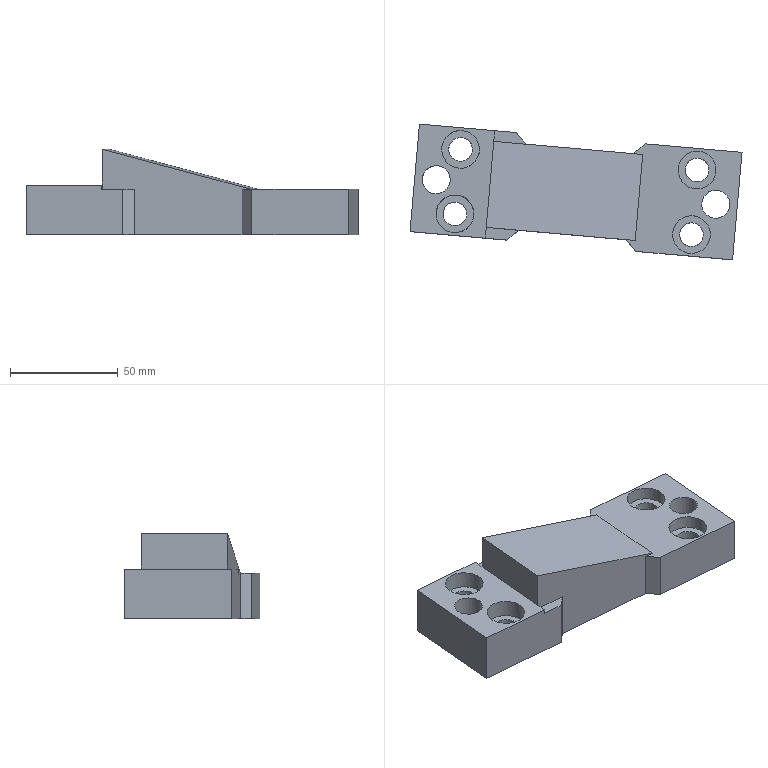Part | NX | features solid 2 | 1 solid | 35 faces | box 153.787 x 62.883 x 39.56 mm | volume 156886 mm3 | plane 25 | cylinder 10 | commonest cylinder face diameters 11 x4 17.5 x4 13 x2
STEP:
#1=CARTESIAN_POINT('',(-568.768,325.811,-44.));
#2=VERTEX_POINT('',#1);
#3=CARTESIAN_POINT('',(-553.825,324.504,-44.));
#4=VERTEX_POINT('',#3);
#5=CARTESIAN_POINT('',(-568.768,325.811,-44.));
#6=DIRECTION('',(0.9962,-0.08716,0.));
#7=VECTOR('',#6,1000.);
#8=LINE('',#5,#7);
#9=EDGE_CURVE('',#2,#4,#8,.T.);
#10=ORIENTED_EDGE('',*,*,#9,.T.);
#11=CARTESIAN_POINT('',(-558.37,329.921,-44.));
#12=VERTEX_POINT('',#11);
#13=CARTESIAN_POINT('',(-553.825,324.504,-44.));
#14=DIRECTION('',(-0.6428,0.766,0.));
#15=VECTOR('',#14,1000.);
#16=LINE('',#13,#15);
#17=EDGE_CURVE('',#4,#12,#16,.T.);
#18=ORIENTED_EDGE('',*,*,#17,.T.);
#19=CARTESIAN_POINT('',(-568.332,330.792,-44.));
#20=VERTEX_POINT('',#19);
#21=CARTESIAN_POINT('',(-603.199,333.843,-44.));
#22=DIRECTION('',(0.9962,-0.08716,0.));
#23=VECTOR('',#22,1000.);
#24=LINE('',#21,#23);
#25=EDGE_CURVE('',#20,#12,#24,.T.);
#26=ORIENTED_EDGE('',*,*,#25,.F.);
#27=CARTESIAN_POINT('',(-572.69,280.982,-44.));
#28=DIRECTION('',(0.08716,0.9962,0.));
#29=VECTOR('',#28,1000.);
#30=LINE('',#27,#29);
#31=EDGE_CURVE('',#2,#20,#30,.T.);
#32=ORIENTED_EDGE('',*,*,#31,.F.);
#33=EDGE_LOOP('',(#10,#18,#26,#32));
#34=FACE_BOUND('',#33,.T.);
#35=CARTESIAN_POINT('',(-607.557,284.033,-44.));
#36=DIRECTION('',(0.,0.,-1.));
#37=DIRECTION('',(-0.08716,-0.9962,0.));
#38=AXIS2_PLACEMENT_3D('',#35,#36,#37);
#39=PLANE('',#38);
#40=ADVANCED_FACE('',(#34),#39,.F.);
#41=CARTESIAN_POINT('',(-572.69,280.982,-44.));
#42=VERTEX_POINT('',#41);
#43=CARTESIAN_POINT('',(-572.254,285.963,-44.));
#44=VERTEX_POINT('',#43);
#45=CARTESIAN_POINT('',(-572.69,280.982,-44.));
#46=DIRECTION('',(0.08716,0.9962,0.));
#47=VECTOR('',#46,1000.);
#48=LINE('',#45,#47);
#49=EDGE_CURVE('',#42,#44,#48,.T.);
#50=ORIENTED_EDGE('',*,*,#49,.F.);
#51=CARTESIAN_POINT('',(-562.728,280.111,-44.));
#52=VERTEX_POINT('',#51);
#53=CARTESIAN_POINT('',(-607.557,284.033,-44.));
#54=DIRECTION('',(0.9962,-0.08716,0.));
#55=VECTOR('',#54,1000.);
#56=LINE('',#53,#55);
#57=EDGE_CURVE('',#42,#52,#56,.T.);
#58=ORIENTED_EDGE('',*,*,#57,.T.);
#59=CARTESIAN_POINT('',(-557.311,284.656,-44.));
#60=VERTEX_POINT('',#59);
#61=CARTESIAN_POINT('',(-562.728,280.111,-44.));
#62=DIRECTION('',(0.766,0.6428,0.));
#63=VECTOR('',#62,1000.);
#64=LINE('',#61,#63);
#65=EDGE_CURVE('',#52,#60,#64,.T.);
#66=ORIENTED_EDGE('',*,*,#65,.T.);
#67=CARTESIAN_POINT('',(-572.254,285.963,-44.));
#68=DIRECTION('',(0.9962,-0.08716,0.));
#69=VECTOR('',#68,1000.);
#70=LINE('',#67,#69);
#71=EDGE_CURVE('',#44,#60,#70,.T.);
#72=ORIENTED_EDGE('',*,*,#71,.F.);
#73=EDGE_LOOP('',(#50,#58,#66,#72));
#74=FACE_BOUND('',#73,.T.);
#75=CARTESIAN_POINT('',(-607.557,284.033,-44.));
#76=DIRECTION('',(0.,0.,-1.));
#77=DIRECTION('',(-0.08716,-0.9962,0.));
#78=AXIS2_PLACEMENT_3D('',#75,#76,#77);
#79=PLANE('',#78);
#80=ADVANCED_FACE('',(#74),#79,.F.);
#81=ORIENTED_EDGE('',*,*,#31,.T.);
#82=CARTESIAN_POINT('',(-568.332,330.792,-42.));
#83=VERTEX_POINT('',#82);
#84=CARTESIAN_POINT('',(-568.332,330.792,-44.));
#85=DIRECTION('',(0.,0.,-1.));
#86=VECTOR('',#85,1000.);
#87=LINE('',#84,#86);
#88=EDGE_CURVE('',#83,#20,#87,.T.);
#89=ORIENTED_EDGE('',*,*,#88,.F.);
#90=CARTESIAN_POINT('',(-568.768,325.811,-42.));
#91=VERTEX_POINT('',#90);
#92=CARTESIAN_POINT('',(-572.69,280.982,-42.));
#93=DIRECTION('',(0.08716,0.9962,0.));
#94=VECTOR('',#93,1000.);
#95=LINE('',#92,#94);
#96=EDGE_CURVE('',#91,#83,#95,.T.);
#97=ORIENTED_EDGE('',*,*,#96,.F.);
#98=CARTESIAN_POINT('',(-568.768,325.811,-25.44));
#99=DIRECTION('',(0.,0.,-1.));
#100=VECTOR('',#99,1000.);
#101=LINE('',#98,#100);
#102=EDGE_CURVE('',#91,#2,#101,.T.);
#103=ORIENTED_EDGE('',*,*,#102,.T.);
#104=EDGE_LOOP('',(#81,#89,#97,#103));
#105=FACE_BOUND('',#104,.T.);
#106=CARTESIAN_POINT('',(-572.69,280.982,-25.44));
#107=DIRECTION('',(0.9962,-0.08716,0.));
#108=DIRECTION('',(-0.08716,-0.9962,0.));
#109=AXIS2_PLACEMENT_3D('',#106,#107,#108);
#110=PLANE('',#109);
#111=ADVANCED_FACE('',(#105),#110,.T.);
#112=CARTESIAN_POINT('',(-468.463,281.902,-44.));
#113=VERTEX_POINT('',#112);
#114=CARTESIAN_POINT('',(-477.18,282.665,-44.));
#115=DIRECTION('',(0.,0.,-1.));
#116=DIRECTION('',(0.9962,-0.08716,0.));
#117=AXIS2_PLACEMENT_3D('',#114,#115,#116);
#118=CIRCLE('',#117,8.75);
#119=EDGE_CURVE('',#113,#113,#118,.T.);
#120=ORIENTED_EDGE('',*,*,#119,.T.);
#121=EDGE_LOOP('',(#120));
#122=FACE_BOUND('',#121,.T.);
#123=CARTESIAN_POINT('',(-507.502,280.298,-44.));
#124=VERTEX_POINT('',#123);
#125=CARTESIAN_POINT('',(-502.956,274.882,-44.));
#126=VERTEX_POINT('',#125);
#127=CARTESIAN_POINT('',(-507.502,280.298,-44.));
#128=DIRECTION('',(0.6428,-0.766,0.));
#129=VECTOR('',#128,1000.);
#130=LINE('',#127,#129);
#131=EDGE_CURVE('',#124,#126,#130,.T.);
#132=ORIENTED_EDGE('',*,*,#131,.T.);
#133=CARTESIAN_POINT('',(-458.128,270.96,-44.));
#134=VERTEX_POINT('',#133);
#135=CARTESIAN_POINT('',(-502.956,274.882,-44.));
#136=DIRECTION('',(0.9962,-0.08716,0.));
#137=VECTOR('',#136,1000.);
#138=LINE('',#135,#137);
#139=EDGE_CURVE('',#126,#134,#138,.T.);
#140=ORIENTED_EDGE('',*,*,#139,.T.);
#141=CARTESIAN_POINT('',(-453.77,320.769,-44.));
#142=VERTEX_POINT('',#141);
#143=CARTESIAN_POINT('',(-458.128,270.96,-44.));
#144=DIRECTION('',(0.08716,0.9962,0.));
#145=VECTOR('',#144,1000.);
#146=LINE('',#143,#145);
#147=EDGE_CURVE('',#134,#142,#146,.T.);
#148=ORIENTED_EDGE('',*,*,#147,.T.);
#149=CARTESIAN_POINT('',(-498.599,324.691,-44.));
#150=VERTEX_POINT('',#149);
#151=CARTESIAN_POINT('',(-498.599,324.691,-44.));
#152=DIRECTION('',(0.9962,-0.08716,0.));
#153=VECTOR('',#152,1000.);
#154=LINE('',#151,#153);
#155=EDGE_CURVE('',#150,#142,#154,.T.);
#156=ORIENTED_EDGE('',*,*,#155,.F.);
#157=CARTESIAN_POINT('',(-504.015,320.146,-44.));
#158=VERTEX_POINT('',#157);
#159=CARTESIAN_POINT('',(-504.015,320.146,-44.));
#160=DIRECTION('',(0.766,0.6428,0.));
#161=VECTOR('',#160,1000.);
#162=LINE('',#159,#161);
#163=EDGE_CURVE('',#158,#150,#162,.T.);
#164=ORIENTED_EDGE('',*,*,#163,.F.);
#165=CARTESIAN_POINT('',(-499.764,319.774,-44.));
#166=VERTEX_POINT('',#165);
#167=CARTESIAN_POINT('',(-568.768,325.811,-44.));
#168=DIRECTION('',(0.9962,-0.08716,0.));
#169=VECTOR('',#168,1000.);
#170=LINE('',#167,#169);
#171=EDGE_CURVE('',#158,#166,#170,.T.);
#172=ORIENTED_EDGE('',*,*,#171,.T.);
#173=CARTESIAN_POINT('',(-503.25,279.926,-44.));
#174=VERTEX_POINT('',#173);
#175=CARTESIAN_POINT('',(-503.25,279.926,-44.));
#176=DIRECTION('',(0.08716,0.9962,0.));
#177=VECTOR('',#176,1000.);
#178=LINE('',#175,#177);
#179=EDGE_CURVE('',#174,#166,#178,.T.);
#180=ORIENTED_EDGE('',*,*,#179,.F.);
#181=CARTESIAN_POINT('',(-572.254,285.963,-44.));
#182=DIRECTION('',(0.9962,-0.08716,0.));
#183=VECTOR('',#182,1000.);
#184=LINE('',#181,#183);
#185=EDGE_CURVE('',#124,#174,#184,.T.);
#186=ORIENTED_EDGE('',*,*,#185,.F.);
#187=EDGE_LOOP('',(#132,#140,#148,#156,#164,#172,#180,#186));
#188=FACE_BOUND('',#187,.T.);
#189=CARTESIAN_POINT('',(-459.435,296.169,-44.));
#190=VERTEX_POINT('',#189);
#191=CARTESIAN_POINT('',(-465.911,296.736,-44.));
#192=DIRECTION('',(0.,0.,-1.));
#193=DIRECTION('',(0.9962,-0.08716,0.));
#194=AXIS2_PLACEMENT_3D('',#191,#192,#193);
#195=CIRCLE('',#194,6.5);
#196=EDGE_CURVE('',#190,#190,#195,.T.);
#197=ORIENTED_EDGE('',*,*,#196,.T.);
#198=EDGE_LOOP('',(#197));
#199=FACE_BOUND('',#198,.T.);
#200=CARTESIAN_POINT('',(-465.849,311.788,-44.));
#201=VERTEX_POINT('',#200);
#202=CARTESIAN_POINT('',(-474.565,312.55,-44.));
#203=DIRECTION('',(0.,0.,-1.));
#204=DIRECTION('',(0.9962,-0.08716,0.));
#205=AXIS2_PLACEMENT_3D('',#202,#203,#204);
#206=CIRCLE('',#205,8.75);
#207=EDGE_CURVE('',#201,#201,#206,.T.);
#208=ORIENTED_EDGE('',*,*,#207,.T.);
#209=EDGE_LOOP('',(#208));
#210=FACE_BOUND('',#209,.T.);
#211=CARTESIAN_POINT('',(-607.557,284.033,-44.));
#212=DIRECTION('',(0.,0.,-1.));
#213=DIRECTION('',(-0.08716,-0.9962,0.));
#214=AXIS2_PLACEMENT_3D('',#211,#212,#213);
#215=PLANE('',#214);
#216=ADVANCED_FACE('',(#122,#188,#199,#210),#215,.F.);
#217=CARTESIAN_POINT('',(-469.086,312.071,-65.));
#218=VERTEX_POINT('',#217);
#219=CARTESIAN_POINT('',(-474.565,312.55,-65.));
#220=DIRECTION('',(0.,0.,-1.));
#221=DIRECTION('',(0.9962,-0.08716,0.));
#222=AXIS2_PLACEMENT_3D('',#219,#220,#221);
#223=CIRCLE('',#222,5.5);
#224=EDGE_CURVE('',#218,#218,#223,.T.);
#225=ORIENTED_EDGE('',*,*,#224,.T.);
#226=EDGE_LOOP('',(#225));
#227=FACE_BOUND('',#226,.T.);
#228=CARTESIAN_POINT('',(-474.086,318.03,-50.));
#229=VERTEX_POINT('',#228);
#230=CARTESIAN_POINT('',(-474.565,312.55,-50.));
#231=DIRECTION('',(0.,0.,-1.));
#232=DIRECTION('',(0.08716,0.9962,0.));
#233=AXIS2_PLACEMENT_3D('',#230,#231,#232);
#234=CIRCLE('',#233,5.5);
#235=EDGE_CURVE('',#229,#229,#234,.T.);
#236=ORIENTED_EDGE('',*,*,#235,.F.);
#237=EDGE_LOOP('',(#236));
#238=FACE_BOUND('',#237,.T.);
#239=CARTESIAN_POINT('',(-474.565,312.55,-44.));
#240=DIRECTION('',(0.,0.,-1.));
#241=DIRECTION('',(-0.08716,-0.9962,0.));
#242=AXIS2_PLACEMENT_3D('',#239,#240,#241);
#243=CYLINDRICAL_SURFACE('',#242,5.5);
#244=ADVANCED_FACE('',(#227,#238),#243,.F.);
#245=CARTESIAN_POINT('',(-471.701,282.185,-65.));
#246=VERTEX_POINT('',#245);
#247=CARTESIAN_POINT('',(-477.18,282.665,-65.));
#248=DIRECTION('',(0.,0.,-1.));
#249=DIRECTION('',(0.9962,-0.08716,0.));
#250=AXIS2_PLACEMENT_3D('',#247,#248,#249);
#251=CIRCLE('',#250,5.5);
#252=EDGE_CURVE('',#246,#246,#251,.T.);
#253=ORIENTED_EDGE('',*,*,#252,.T.);
#254=EDGE_LOOP('',(#253));
#255=FACE_BOUND('',#254,.T.);
#256=CARTESIAN_POINT('',(-476.701,288.144,-50.));
#257=VERTEX_POINT('',#256);
#258=CARTESIAN_POINT('',(-477.18,282.665,-50.));
#259=DIRECTION('',(0.,0.,-1.));
#260=DIRECTION('',(0.08716,0.9962,0.));
#261=AXIS2_PLACEMENT_3D('',#258,#259,#260);
#262=CIRCLE('',#261,5.5);
#263=EDGE_CURVE('',#257,#257,#262,.T.);
#264=ORIENTED_EDGE('',*,*,#263,.F.);
#265=EDGE_LOOP('',(#264));
#266=FACE_BOUND('',#265,.T.);
#267=CARTESIAN_POINT('',(-477.18,282.665,-44.));
#268=DIRECTION('',(0.,0.,-1.));
#269=DIRECTION('',(-0.08716,-0.9962,0.));
#270=AXIS2_PLACEMENT_3D('',#267,#268,#269);
#271=CYLINDRICAL_SURFACE('',#270,5.5);
#272=ADVANCED_FACE('',(#255,#266),#271,.F.);
#273=CARTESIAN_POINT('',(-603.199,333.843,-65.));
#274=VERTEX_POINT('',#273);
#275=CARTESIAN_POINT('',(-558.37,329.921,-65.));
#276=VERTEX_POINT('',#275);
#277=CARTESIAN_POINT('',(-603.199,333.843,-65.));
#278=DIRECTION('',(0.9962,-0.08716,0.));
#279=VECTOR('',#278,1000.);
#280=LINE('',#277,#279);
#281=EDGE_CURVE('',#274,#276,#280,.T.);
#282=ORIENTED_EDGE('',*,*,#281,.T.);
#283=CARTESIAN_POINT('',(-553.825,324.504,-65.));
#284=VERTEX_POINT('',#283);
#285=CARTESIAN_POINT('',(-553.825,324.504,-65.));
#286=DIRECTION('',(-0.6428,0.766,0.));
#287=VECTOR('',#286,1000.);
#288=LINE('',#285,#287);
#289=EDGE_CURVE('',#284,#276,#288,.T.);
#290=ORIENTED_EDGE('',*,*,#289,.F.);
#291=CARTESIAN_POINT('',(-504.015,320.146,-65.));
#292=VERTEX_POINT('',#291);
#293=CARTESIAN_POINT('',(-553.825,324.504,-65.));
#294=DIRECTION('',(0.9962,-0.08716,0.));
#295=VECTOR('',#294,1000.);
#296=LINE('',#293,#295);
#297=EDGE_CURVE('',#284,#292,#296,.T.);
#298=ORIENTED_EDGE('',*,*,#297,.T.);
#299=CARTESIAN_POINT('',(-498.599,324.691,-65.));
#300=VERTEX_POINT('',#299);
#301=CARTESIAN_POINT('',(-504.015,320.146,-65.));
#302=DIRECTION('',(0.766,0.6428,0.));
#303=VECTOR('',#302,1000.);
#304=LINE('',#301,#303);
#305=EDGE_CURVE('',#292,#300,#304,.T.);
#306=ORIENTED_EDGE('',*,*,#305,.T.);
#307=CARTESIAN_POINT('',(-453.77,320.769,-65.));
#308=VERTEX_POINT('',#307);
#309=CARTESIAN_POINT('',(-498.599,324.691,-65.));
#310=DIRECTION('',(0.9962,-0.08716,0.));
#311=VECTOR('',#310,1000.);
#312=LINE('',#309,#311);
#313=EDGE_CURVE('',#300,#308,#312,.T.);
#314=ORIENTED_EDGE('',*,*,#313,.T.);
#315=CARTESIAN_POINT('',(-458.128,270.96,-65.));
#316=VERTEX_POINT('',#315);
#317=CARTESIAN_POINT('',(-458.128,270.96,-65.));
#318=DIRECTION('',(0.08716,0.9962,0.));
#319=VECTOR('',#318,1000.);
#320=LINE('',#317,#319);
#321=EDGE_CURVE('',#316,#308,#320,.T.);
#322=ORIENTED_EDGE('',*,*,#321,.F.);
#323=CARTESIAN_POINT('',(-502.956,274.882,-65.));
#324=VERTEX_POINT('',#323);
#325=CARTESIAN_POINT('',(-502.956,274.882,-65.));
#326=DIRECTION('',(0.9962,-0.08716,0.));
#327=VECTOR('',#326,1000.);
#328=LINE('',#325,#327);
#329=EDGE_CURVE('',#324,#316,#328,.T.);
#330=ORIENTED_EDGE('',*,*,#329,.F.);
#331=CARTESIAN_POINT('',(-507.502,280.298,-65.));
#332=VERTEX_POINT('',#331);
#333=CARTESIAN_POINT('',(-507.502,280.298,-65.));
#334=DIRECTION('',(0.6428,-0.766,0.));
#335=VECTOR('',#334,1000.);
#336=LINE('',#333,#335);
#337=EDGE_CURVE('',#332,#324,#336,.T.);
#338=ORIENTED_EDGE('',*,*,#337,.F.);
#339=CARTESIAN_POINT('',(-557.311,284.656,-65.));
#340=VERTEX_POINT('',#339);
#341=CARTESIAN_POINT('',(-557.311,284.656,-65.));
#342=DIRECTION('',(0.9962,-0.08716,0.));
#343=VECTOR('',#342,1000.);
#344=LINE('',#341,#343);
#345=EDGE_CURVE('',#340,#332,#344,.T.);
#346=ORIENTED_EDGE('',*,*,#345,.F.);
#347=CARTESIAN_POINT('',(-562.728,280.111,-65.));
#348=VERTEX_POINT('',#347);
#349=CARTESIAN_POINT('',(-562.728,280.111,-65.));
#350=DIRECTION('',(0.766,0.6428,0.));
#351=VECTOR('',#350,1000.);
#352=LINE('',#349,#351);
#353=EDGE_CURVE('',#348,#340,#352,.T.);
#354=ORIENTED_EDGE('',*,*,#353,.F.);
#355=CARTESIAN_POINT('',(-607.557,284.033,-65.));
#356=VERTEX_POINT('',#355);
#357=CARTESIAN_POINT('',(-607.557,284.033,-65.));
#358=DIRECTION('',(0.9962,-0.08716,0.));
#359=VECTOR('',#358,1000.);
#360=LINE('',#357,#359);
#361=EDGE_CURVE('',#356,#348,#360,.T.);
#362=ORIENTED_EDGE('',*,*,#361,.F.);
#363=CARTESIAN_POINT('',(-603.199,333.843,-65.));
#364=DIRECTION('',(-0.08716,-0.9962,0.));
#365=VECTOR('',#364,1000.);
#366=LINE('',#363,#365);
#367=EDGE_CURVE('',#274,#356,#366,.T.);
#368=ORIENTED_EDGE('',*,*,#367,.F.);
#369=EDGE_LOOP('',(#282,#290,#298,#306,#314,#322,#330,#338,#346,#354,#362,#368));
#370=FACE_BOUND('',#369,.T.);
#371=ORIENTED_EDGE('',*,*,#224,.F.);
#372=EDGE_LOOP('',(#371));
#373=FACE_BOUND('',#372,.T.);
#374=ORIENTED_EDGE('',*,*,#252,.F.);
#375=EDGE_LOOP('',(#374));
#376=FACE_BOUND('',#375,.T.);
#377=CARTESIAN_POINT('',(-459.435,296.169,-65.));
#378=VERTEX_POINT('',#377);
#379=CARTESIAN_POINT('',(-465.911,296.736,-65.));
#380=DIRECTION('',(0.,0.,-1.));
#381=DIRECTION('',(0.9962,-0.08716,0.));
#382=AXIS2_PLACEMENT_3D('',#379,#380,#381);
#383=CIRCLE('',#382,6.5);
#384=EDGE_CURVE('',#378,#378,#383,.T.);
#385=ORIENTED_EDGE('',*,*,#384,.F.);
#386=EDGE_LOOP('',(#385));
#387=FACE_BOUND('',#386,.T.);
#388=CARTESIAN_POINT('',(-578.668,321.658,-65.));
#389=VERTEX_POINT('',#388);
#390=CARTESIAN_POINT('',(-584.147,322.138,-65.));
#391=DIRECTION('',(0.,0.,-1.));
#392=DIRECTION('',(0.9962,-0.08716,0.));
#393=AXIS2_PLACEMENT_3D('',#390,#391,#392);
#394=CIRCLE('',#393,5.5);
#395=EDGE_CURVE('',#389,#389,#394,.T.);
#396=ORIENTED_EDGE('',*,*,#395,.F.);
#397=EDGE_LOOP('',(#396));
#398=FACE_BOUND('',#397,.T.);
#399=CARTESIAN_POINT('',(-581.282,291.772,-65.));
#400=VERTEX_POINT('',#399);
#401=CARTESIAN_POINT('',(-586.761,292.252,-65.));
#402=DIRECTION('',(0.,0.,-1.));
#403=DIRECTION('',(0.9962,-0.08716,0.));
#404=AXIS2_PLACEMENT_3D('',#401,#402,#403);
#405=CIRCLE('',#404,5.5);
#406=EDGE_CURVE('',#400,#400,#405,.T.);
#407=ORIENTED_EDGE('',*,*,#406,.F.);
#408=EDGE_LOOP('',(#407));
#409=FACE_BOUND('',#408,.T.);
#410=CARTESIAN_POINT('',(-588.941,307.5,-65.));
#411=VERTEX_POINT('',#410);
#412=CARTESIAN_POINT('',(-595.416,308.066,-65.));
#413=DIRECTION('',(0.,0.,-1.));
#414=DIRECTION('',(0.9962,-0.08716,0.));
#415=AXIS2_PLACEMENT_3D('',#412,#413,#414);
#416=CIRCLE('',#415,6.5);
#417=EDGE_CURVE('',#411,#411,#416,.T.);
#418=ORIENTED_EDGE('',*,*,#417,.F.);
#419=EDGE_LOOP('',(#418));
#420=FACE_BOUND('',#419,.T.);
#421=CARTESIAN_POINT('',(-607.557,284.033,-65.));
#422=DIRECTION('',(0.,0.,-1.));
#423=DIRECTION('',(-0.08716,-0.9962,0.));
#424=AXIS2_PLACEMENT_3D('',#421,#422,#423);
#425=PLANE('',#424);
#426=ADVANCED_FACE('',(#370,#373,#376,#387,#398,#409,#420),#425,.T.);
#427=ORIENTED_EDGE('',*,*,#361,.T.);
#428=CARTESIAN_POINT('',(-562.728,280.111,-44.));
#429=DIRECTION('',(0.,0.,-1.));
#430=VECTOR('',#429,1000.);
#431=LINE('',#428,#430);
#432=EDGE_CURVE('',#52,#348,#431,.T.);
#433=ORIENTED_EDGE('',*,*,#432,.F.);
#434=ORIENTED_EDGE('',*,*,#57,.F.);
#435=CARTESIAN_POINT('',(-572.69,280.982,-42.));
#436=VERTEX_POINT('',#435);
#437=CARTESIAN_POINT('',(-572.69,280.982,-44.));
#438=DIRECTION('',(0.,0.,-1.));
#439=VECTOR('',#438,1000.);
#440=LINE('',#437,#439);
#441=EDGE_CURVE('',#436,#42,#440,.T.);
#442=ORIENTED_EDGE('',*,*,#441,.F.);
#443=CARTESIAN_POINT('',(-607.557,284.033,-42.));
#444=VERTEX_POINT('',#443);
#445=CARTESIAN_POINT('',(-607.557,284.033,-42.));
#446=DIRECTION('',(0.9962,-0.08716,0.));
#447=VECTOR('',#446,1000.);
#448=LINE('',#445,#447);
#449=EDGE_CURVE('',#444,#436,#448,.T.);
#450=ORIENTED_EDGE('',*,*,#449,.F.);
#451=CARTESIAN_POINT('',(-607.557,284.033,-44.));
#452=DIRECTION('',(0.,0.,-1.));
#453=VECTOR('',#452,1000.);
#454=LINE('',#451,#453);
#455=EDGE_CURVE('',#444,#356,#454,.T.);
#456=ORIENTED_EDGE('',*,*,#455,.T.);
#457=EDGE_LOOP('',(#427,#433,#434,#442,#450,#456));
#458=FACE_BOUND('',#457,.T.);
#459=CARTESIAN_POINT('',(-607.557,284.033,-44.));
#460=DIRECTION('',(-0.08716,-0.9962,0.));
#461=DIRECTION('',(-0.9962,0.08716,0.));
#462=AXIS2_PLACEMENT_3D('',#459,#460,#461);
#463=PLANE('',#462);
#464=ADVANCED_FACE('',(#458),#463,.T.);
#465=ORIENTED_EDGE('',*,*,#353,.T.);
#466=CARTESIAN_POINT('',(-557.311,284.656,-44.));
#467=DIRECTION('',(0.,0.,-1.));
#468=VECTOR('',#467,1000.);
#469=LINE('',#466,#468);
#470=EDGE_CURVE('',#60,#340,#469,.T.);
#471=ORIENTED_EDGE('',*,*,#470,.F.);
#472=ORIENTED_EDGE('',*,*,#65,.F.);
#473=ORIENTED_EDGE('',*,*,#432,.T.);
#474=EDGE_LOOP('',(#465,#471,#472,#473));
#475=FACE_BOUND('',#474,.T.);
#476=CARTESIAN_POINT('',(-562.728,280.111,-44.));
#477=DIRECTION('',(0.6428,-0.766,0.));
#478=DIRECTION('',(-0.766,-0.6428,0.));
#479=AXIS2_PLACEMENT_3D('',#476,#477,#478);
#480=PLANE('',#479);
#481=ADVANCED_FACE('',(#475),#480,.T.);
#482=ORIENTED_EDGE('',*,*,#345,.T.);
#483=CARTESIAN_POINT('',(-507.502,280.298,-44.));
#484=DIRECTION('',(0.,0.,-1.));
#485=VECTOR('',#484,1000.);
#486=LINE('',#483,#485);
#487=EDGE_CURVE('',#124,#332,#486,.T.);
#488=ORIENTED_EDGE('',*,*,#487,.F.);
#489=ORIENTED_EDGE('',*,*,#185,.T.);
#490=CARTESIAN_POINT('',(-572.254,285.963,-25.44));
#491=VERTEX_POINT('',#490);
#492=CARTESIAN_POINT('',(-572.254,285.963,-25.44));
#493=DIRECTION('',(0.9623,-0.08419,-0.2588));
#494=VECTOR('',#493,1000.);
#495=LINE('',#492,#494);
#496=EDGE_CURVE('',#491,#174,#495,.T.);
#497=ORIENTED_EDGE('',*,*,#496,.F.);
#498=CARTESIAN_POINT('',(-572.254,285.963,-42.));
#499=VERTEX_POINT('',#498);
#500=CARTESIAN_POINT('',(-572.254,285.963,-25.44));
#501=DIRECTION('',(0.,0.,-1.));
#502=VECTOR('',#501,1000.);
#503=LINE('',#500,#502);
#504=EDGE_CURVE('',#491,#499,#503,.T.);
#505=ORIENTED_EDGE('',*,*,#504,.T.);
#506=CARTESIAN_POINT('',(-572.254,285.963,-25.44));
#507=DIRECTION('',(0.,0.,-1.));
#508=VECTOR('',#507,1000.);
#509=LINE('',#506,#508);
#510=EDGE_CURVE('',#499,#44,#509,.T.);
#511=ORIENTED_EDGE('',*,*,#510,.T.);
#512=ORIENTED_EDGE('',*,*,#71,.T.);
#513=ORIENTED_EDGE('',*,*,#470,.T.);
#514=EDGE_LOOP('',(#482,#488,#489,#497,#505,#511,#512,#513));
#515=FACE_BOUND('',#514,.T.);
#516=CARTESIAN_POINT('',(-557.311,284.656,-44.));
#517=DIRECTION('',(-0.08716,-0.9962,0.));
#518=DIRECTION('',(-0.9962,0.08716,0.));
#519=AXIS2_PLACEMENT_3D('',#516,#517,#518);
#520=PLANE('',#519);
#521=ADVANCED_FACE('',(#515),#520,.T.);
#522=ORIENTED_EDGE('',*,*,#337,.T.);
#523=CARTESIAN_POINT('',(-502.956,274.882,-44.));
#524=DIRECTION('',(0.,0.,-1.));
#525=VECTOR('',#524,1000.);
#526=LINE('',#523,#525);
#527=EDGE_CURVE('',#126,#324,#526,.T.);
#528=ORIENTED_EDGE('',*,*,#527,.F.);
#529=ORIENTED_EDGE('',*,*,#131,.F.);
#530=ORIENTED_EDGE('',*,*,#487,.T.);
#531=EDGE_LOOP('',(#522,#528,#529,#530));
#532=FACE_BOUND('',#531,.T.);
#533=CARTESIAN_POINT('',(-507.502,280.298,-44.));
#534=DIRECTION('',(-0.766,-0.6428,0.));
#535=DIRECTION('',(-0.6428,0.766,0.));
#536=AXIS2_PLACEMENT_3D('',#533,#534,#535);
#537=PLANE('',#536);
#538=ADVANCED_FACE('',(#532),#537,.T.);
#539=ORIENTED_EDGE('',*,*,#329,.T.);
#540=CARTESIAN_POINT('',(-458.128,270.96,-44.));
#541=DIRECTION('',(0.,0.,-1.));
#542=VECTOR('',#541,1000.);
#543=LINE('',#540,#542);
#544=EDGE_CURVE('',#134,#316,#543,.T.);
#545=ORIENTED_EDGE('',*,*,#544,.F.);
#546=ORIENTED_EDGE('',*,*,#139,.F.);
#547=ORIENTED_EDGE('',*,*,#527,.T.);
#548=EDGE_LOOP('',(#539,#545,#546,#547));
#549=FACE_BOUND('',#548,.T.);
#550=CARTESIAN_POINT('',(-502.956,274.882,-44.));
#551=DIRECTION('',(-0.08716,-0.9962,0.));
#552=DIRECTION('',(-0.9962,0.08716,0.));
#553=AXIS2_PLACEMENT_3D('',#550,#551,#552);
#554=PLANE('',#553);
#555=ADVANCED_FACE('',(#549),#554,.T.);
#556=ORIENTED_EDGE('',*,*,#321,.T.);
#557=CARTESIAN_POINT('',(-453.77,320.769,-44.));
#558=DIRECTION('',(0.,0.,-1.));
#559=VECTOR('',#558,1000.);
#560=LINE('',#557,#559);
#561=EDGE_CURVE('',#142,#308,#560,.T.);
#562=ORIENTED_EDGE('',*,*,#561,.F.);
#563=ORIENTED_EDGE('',*,*,#147,.F.);
#564=ORIENTED_EDGE('',*,*,#544,.T.);
#565=EDGE_LOOP('',(#556,#562,#563,#564));
#566=FACE_BOUND('',#565,.T.);
#567=CARTESIAN_POINT('',(-458.128,270.96,-44.));
#568=DIRECTION('',(0.9962,-0.08716,0.));
#569=DIRECTION('',(-0.08716,-0.9962,0.));
#570=AXIS2_PLACEMENT_3D('',#567,#568,#569);
#571=PLANE('',#570);
#572=ADVANCED_FACE('',(#566),#571,.T.);
#573=ORIENTED_EDGE('',*,*,#313,.F.);
#574=CARTESIAN_POINT('',(-498.599,324.691,-44.));
#575=DIRECTION('',(0.,0.,-1.));
#576=VECTOR('',#575,1000.);
#577=LINE('',#574,#576);
#578=EDGE_CURVE('',#150,#300,#577,.T.);
#579=ORIENTED_EDGE('',*,*,#578,.F.);
#580=ORIENTED_EDGE('',*,*,#155,.T.);
#581=ORIENTED_EDGE('',*,*,#561,.T.);
#582=EDGE_LOOP('',(#573,#579,#580,#581));
#583=FACE_BOUND('',#582,.T.);
#584=CARTESIAN_POINT('',(-498.599,324.691,-44.));
#585=DIRECTION('',(-0.08716,-0.9962,0.));
#586=DIRECTION('',(-0.9962,0.08716,0.));
#587=AXIS2_PLACEMENT_3D('',#584,#585,#586);
#588=PLANE('',#587);
#589=ADVANCED_FACE('',(#583),#588,.F.);
#590=ORIENTED_EDGE('',*,*,#305,.F.);
#591=CARTESIAN_POINT('',(-504.015,320.146,-44.));
#592=DIRECTION('',(0.,0.,-1.));
#593=VECTOR('',#592,1000.);
#594=LINE('',#591,#593);
#595=EDGE_CURVE('',#158,#292,#594,.T.);
#596=ORIENTED_EDGE('',*,*,#595,.F.);
#597=ORIENTED_EDGE('',*,*,#163,.T.);
#598=ORIENTED_EDGE('',*,*,#578,.T.);
#599=EDGE_LOOP('',(#590,#596,#597,#598));
#600=FACE_BOUND('',#599,.T.);
#601=CARTESIAN_POINT('',(-504.015,320.146,-44.));
#602=DIRECTION('',(0.6428,-0.766,0.));
#603=DIRECTION('',(-0.766,-0.6428,0.));
#604=AXIS2_PLACEMENT_3D('',#601,#602,#603);
#605=PLANE('',#604);
#606=ADVANCED_FACE('',(#600),#605,.F.);
#607=ORIENTED_EDGE('',*,*,#297,.F.);
#608=CARTESIAN_POINT('',(-553.825,324.504,-44.));
#609=DIRECTION('',(0.,0.,-1.));
#610=VECTOR('',#609,1000.);
#611=LINE('',#608,#610);
#612=EDGE_CURVE('',#4,#284,#611,.T.);
#613=ORIENTED_EDGE('',*,*,#612,.F.);
#614=ORIENTED_EDGE('',*,*,#9,.F.);
#615=ORIENTED_EDGE('',*,*,#102,.F.);
#616=CARTESIAN_POINT('',(-568.768,325.811,-25.44));
#617=VERTEX_POINT('',#616);
#618=CARTESIAN_POINT('',(-568.768,325.811,-25.44));
#619=DIRECTION('',(0.,0.,-1.));
#620=VECTOR('',#619,1000.);
#621=LINE('',#618,#620);
#622=EDGE_CURVE('',#617,#91,#621,.T.);
#623=ORIENTED_EDGE('',*,*,#622,.F.);
#624=CARTESIAN_POINT('',(-568.768,325.811,-25.44));
#625=DIRECTION('',(0.9623,-0.08419,-0.2588));
#626=VECTOR('',#625,1000.);
#627=LINE('',#624,#626);
#628=EDGE_CURVE('',#617,#166,#627,.T.);
#629=ORIENTED_EDGE('',*,*,#628,.T.);
#630=ORIENTED_EDGE('',*,*,#171,.F.);
#631=ORIENTED_EDGE('',*,*,#595,.T.);
#632=EDGE_LOOP('',(#607,#613,#614,#615,#623,#629,#630,#631));
#633=FACE_BOUND('',#632,.T.);
#634=CARTESIAN_POINT('',(-553.825,324.504,-44.));
#635=DIRECTION('',(-0.08716,-0.9962,0.));
#636=DIRECTION('',(-0.9962,0.08716,0.));
#637=AXIS2_PLACEMENT_3D('',#634,#635,#636);
#638=PLANE('',#637);
#639=ADVANCED_FACE('',(#633),#638,.F.);
#640=ORIENTED_EDGE('',*,*,#289,.T.);
#641=CARTESIAN_POINT('',(-558.37,329.921,-44.));
#642=DIRECTION('',(0.,0.,-1.));
#643=VECTOR('',#642,1000.);
#644=LINE('',#641,#643);
#645=EDGE_CURVE('',#12,#276,#644,.T.);
#646=ORIENTED_EDGE('',*,*,#645,.F.);
#647=ORIENTED_EDGE('',*,*,#17,.F.);
#648=ORIENTED_EDGE('',*,*,#612,.T.);
#649=EDGE_LOOP('',(#640,#646,#647,#648));
#650=FACE_BOUND('',#649,.T.);
#651=CARTESIAN_POINT('',(-553.825,324.504,-44.));
#652=DIRECTION('',(0.766,0.6428,0.));
#653=DIRECTION('',(0.6428,-0.766,0.));
#654=AXIS2_PLACEMENT_3D('',#651,#652,#653);
#655=PLANE('',#654);
#656=ADVANCED_FACE('',(#650),#655,.T.);
#657=ORIENTED_EDGE('',*,*,#25,.T.);
#658=ORIENTED_EDGE('',*,*,#645,.T.);
#659=ORIENTED_EDGE('',*,*,#281,.F.);
#660=CARTESIAN_POINT('',(-603.199,333.843,-42.));
#661=VERTEX_POINT('',#660);
#662=CARTESIAN_POINT('',(-603.199,333.843,-44.));
#663=DIRECTION('',(0.,0.,-1.));
#664=VECTOR('',#663,1000.);
#665=LINE('',#662,#664);
#666=EDGE_CURVE('',#661,#274,#665,.T.);
#667=ORIENTED_EDGE('',*,*,#666,.F.);
#668=CARTESIAN_POINT('',(-603.199,333.843,-42.));
#669=DIRECTION('',(0.9962,-0.08716,0.));
#670=VECTOR('',#669,1000.);
#671=LINE('',#668,#670);
#672=EDGE_CURVE('',#661,#83,#671,.T.);
#673=ORIENTED_EDGE('',*,*,#672,.T.);
#674=ORIENTED_EDGE('',*,*,#88,.T.);
#675=EDGE_LOOP('',(#657,#658,#659,#667,#673,#674));
#676=FACE_BOUND('',#675,.T.);
#677=CARTESIAN_POINT('',(-603.199,333.843,-44.));
#678=DIRECTION('',(-0.08716,-0.9962,0.));
#679=DIRECTION('',(-0.9962,0.08716,0.));
#680=AXIS2_PLACEMENT_3D('',#677,#678,#679);
#681=PLANE('',#680);
#682=ADVANCED_FACE('',(#676),#681,.F.);
#683=ORIENTED_EDGE('',*,*,#196,.F.);
#684=EDGE_LOOP('',(#683));
#685=FACE_BOUND('',#684,.T.);
#686=ORIENTED_EDGE('',*,*,#384,.T.);
#687=EDGE_LOOP('',(#686));
#688=FACE_BOUND('',#687,.T.);
#689=CARTESIAN_POINT('',(-465.911,296.736,-44.));
#690=DIRECTION('',(0.,0.,-1.));
#691=DIRECTION('',(-0.08716,-0.9962,0.));
#692=AXIS2_PLACEMENT_3D('',#689,#690,#691);
#693=CYLINDRICAL_SURFACE('',#692,6.5);
#694=ADVANCED_FACE('',(#685,#688),#693,.F.);
#695=ORIENTED_EDGE('',*,*,#119,.F.);
#696=EDGE_LOOP('',(#695));
#697=FACE_BOUND('',#696,.T.);
#698=CARTESIAN_POINT('',(-468.463,281.902,-50.));
#699=VERTEX_POINT('',#698);
#700=CARTESIAN_POINT('',(-477.18,282.665,-50.));
#701=DIRECTION('',(0.,0.,-1.));
#702=DIRECTION('',(0.9962,-0.08716,0.));
#703=AXIS2_PLACEMENT_3D('',#700,#701,#702);
#704=CIRCLE('',#703,8.75);
#705=EDGE_CURVE('',#699,#699,#704,.T.);
#706=ORIENTED_EDGE('',*,*,#705,.T.);
#707=EDGE_LOOP('',(#706));
#708=FACE_BOUND('',#707,.T.);
#709=CARTESIAN_POINT('',(-477.18,282.665,-44.));
#710=DIRECTION('',(0.,0.,-1.));
#711=DIRECTION('',(-0.08716,-0.9962,0.));
#712=AXIS2_PLACEMENT_3D('',#709,#710,#711);
#713=CYLINDRICAL_SURFACE('',#712,8.75);
#714=ADVANCED_FACE('',(#697,#708),#713,.F.);
#715=ORIENTED_EDGE('',*,*,#263,.T.);
#716=EDGE_LOOP('',(#715));
#717=FACE_BOUND('',#716,.T.);
#718=ORIENTED_EDGE('',*,*,#705,.F.);
#719=EDGE_LOOP('',(#718));
#720=FACE_BOUND('',#719,.T.);
#721=CARTESIAN_POINT('',(-477.18,282.665,-50.));
#722=DIRECTION('',(0.,0.,1.));
#723=DIRECTION('',(0.08716,0.9962,0.));
#724=AXIS2_PLACEMENT_3D('',#721,#722,#723);
#725=PLANE('',#724);
#726=ADVANCED_FACE('',(#717,#720),#725,.T.);
#727=ORIENTED_EDGE('',*,*,#207,.F.);
#728=EDGE_LOOP('',(#727));
#729=FACE_BOUND('',#728,.T.);
#730=CARTESIAN_POINT('',(-465.849,311.788,-50.));
#731=VERTEX_POINT('',#730);
#732=CARTESIAN_POINT('',(-474.565,312.55,-50.));
#733=DIRECTION('',(0.,0.,-1.));
#734=DIRECTION('',(0.9962,-0.08716,0.));
#735=AXIS2_PLACEMENT_3D('',#732,#733,#734);
#736=CIRCLE('',#735,8.75);
#737=EDGE_CURVE('',#731,#731,#736,.T.);
#738=ORIENTED_EDGE('',*,*,#737,.T.);
#739=EDGE_LOOP('',(#738));
#740=FACE_BOUND('',#739,.T.);
#741=CARTESIAN_POINT('',(-474.565,312.55,-44.));
#742=DIRECTION('',(0.,0.,-1.));
#743=DIRECTION('',(-0.08716,-0.9962,0.));
#744=AXIS2_PLACEMENT_3D('',#741,#742,#743);
#745=CYLINDRICAL_SURFACE('',#744,8.75);
#746=ADVANCED_FACE('',(#729,#740),#745,.F.);
#747=ORIENTED_EDGE('',*,*,#235,.T.);
#748=EDGE_LOOP('',(#747));
#749=FACE_BOUND('',#748,.T.);
#750=ORIENTED_EDGE('',*,*,#737,.F.);
#751=EDGE_LOOP('',(#750));
#752=FACE_BOUND('',#751,.T.);
#753=CARTESIAN_POINT('',(-474.565,312.55,-50.));
#754=DIRECTION('',(0.,0.,1.));
#755=DIRECTION('',(0.08716,0.9962,0.));
#756=AXIS2_PLACEMENT_3D('',#753,#754,#755);
#757=PLANE('',#756);
#758=ADVANCED_FACE('',(#749,#752),#757,.T.);
#759=ORIENTED_EDGE('',*,*,#510,.F.);
#760=CARTESIAN_POINT('',(-572.69,280.982,-42.));
#761=DIRECTION('',(0.08716,0.9962,0.));
#762=VECTOR('',#761,1000.);
#763=LINE('',#760,#762);
#764=EDGE_CURVE('',#436,#499,#763,.T.);
#765=ORIENTED_EDGE('',*,*,#764,.F.);
#766=ORIENTED_EDGE('',*,*,#441,.T.);
#767=ORIENTED_EDGE('',*,*,#49,.T.);
#768=EDGE_LOOP('',(#759,#765,#766,#767));
#769=FACE_BOUND('',#768,.T.);
#770=CARTESIAN_POINT('',(-572.69,280.982,-25.44));
#771=DIRECTION('',(0.9962,-0.08716,0.));
#772=DIRECTION('',(-0.08716,-0.9962,0.));
#773=AXIS2_PLACEMENT_3D('',#770,#771,#772);
#774=PLANE('',#773);
#775=ADVANCED_FACE('',(#769),#774,.T.);
#776=CARTESIAN_POINT('',(-586.282,297.731,-50.));
#777=VERTEX_POINT('',#776);
#778=CARTESIAN_POINT('',(-586.761,292.252,-50.));
#779=DIRECTION('',(0.,0.,-1.));
#780=DIRECTION('',(0.08716,0.9962,0.));
#781=AXIS2_PLACEMENT_3D('',#778,#779,#780);
#782=CIRCLE('',#781,5.5);
#783=EDGE_CURVE('',#777,#777,#782,.T.);
#784=ORIENTED_EDGE('',*,*,#783,.T.);
#785=EDGE_LOOP('',(#784));
#786=FACE_BOUND('',#785,.T.);
#787=CARTESIAN_POINT('',(-578.045,291.489,-50.));
#788=VERTEX_POINT('',#787);
#789=CARTESIAN_POINT('',(-586.761,292.252,-50.));
#790=DIRECTION('',(0.,0.,-1.));
#791=DIRECTION('',(0.9962,-0.08716,0.));
#792=AXIS2_PLACEMENT_3D('',#789,#790,#791);
#793=CIRCLE('',#792,8.75);
#794=EDGE_CURVE('',#788,#788,#793,.T.);
#795=ORIENTED_EDGE('',*,*,#794,.F.);
#796=EDGE_LOOP('',(#795));
#797=FACE_BOUND('',#796,.T.);
#798=CARTESIAN_POINT('',(-586.761,292.252,-50.));
#799=DIRECTION('',(0.,0.,1.));
#800=DIRECTION('',(0.08716,0.9962,0.));
#801=AXIS2_PLACEMENT_3D('',#798,#799,#800);
#802=PLANE('',#801);
#803=ADVANCED_FACE('',(#786,#797),#802,.T.);
#804=CARTESIAN_POINT('',(-583.667,327.617,-50.));
#805=VERTEX_POINT('',#804);
#806=CARTESIAN_POINT('',(-584.147,322.138,-50.));
#807=DIRECTION('',(0.,0.,-1.));
#808=DIRECTION('',(0.08716,0.9962,0.));
#809=AXIS2_PLACEMENT_3D('',#806,#807,#808);
#810=CIRCLE('',#809,5.5);
#811=EDGE_CURVE('',#805,#805,#810,.T.);
#812=ORIENTED_EDGE('',*,*,#811,.T.);
#813=EDGE_LOOP('',(#812));
#814=FACE_BOUND('',#813,.T.);
#815=CARTESIAN_POINT('',(-575.43,321.375,-50.));
#816=VERTEX_POINT('',#815);
#817=CARTESIAN_POINT('',(-584.147,322.138,-50.));
#818=DIRECTION('',(0.,0.,-1.));
#819=DIRECTION('',(0.9962,-0.08716,0.));
#820=AXIS2_PLACEMENT_3D('',#817,#818,#819);
#821=CIRCLE('',#820,8.75);
#822=EDGE_CURVE('',#816,#816,#821,.T.);
#823=ORIENTED_EDGE('',*,*,#822,.F.);
#824=EDGE_LOOP('',(#823));
#825=FACE_BOUND('',#824,.T.);
#826=CARTESIAN_POINT('',(-584.147,322.138,-50.));
#827=DIRECTION('',(0.,0.,1.));
#828=DIRECTION('',(0.08716,0.9962,0.));
#829=AXIS2_PLACEMENT_3D('',#826,#827,#828);
#830=PLANE('',#829);
#831=ADVANCED_FACE('',(#814,#825),#830,.T.);
#832=CARTESIAN_POINT('',(-587.524,283.535,-42.));
#833=VERTEX_POINT('',#832);
#834=CARTESIAN_POINT('',(-586.761,292.252,-42.));
#835=DIRECTION('',(0.,0.,1.));
#836=DIRECTION('',(-0.08716,-0.9962,0.));
#837=AXIS2_PLACEMENT_3D('',#834,#835,#836);
#838=CIRCLE('',#837,8.75);
#839=EDGE_CURVE('',#833,#833,#838,.F.);
#840=ORIENTED_EDGE('',*,*,#839,.F.);
#841=EDGE_LOOP('',(#840));
#842=FACE_BOUND('',#841,.T.);
#843=ORIENTED_EDGE('',*,*,#794,.T.);
#844=EDGE_LOOP('',(#843));
#845=FACE_BOUND('',#844,.T.);
#846=CARTESIAN_POINT('',(-586.761,292.252,-44.));
#847=DIRECTION('',(0.,0.,-1.));
#848=DIRECTION('',(-0.08716,-0.9962,0.));
#849=AXIS2_PLACEMENT_3D('',#846,#847,#848);
#850=CYLINDRICAL_SURFACE('',#849,8.75);
#851=ADVANCED_FACE('',(#842,#845),#850,.F.);
#852=CARTESIAN_POINT('',(-584.909,313.421,-42.));
#853=VERTEX_POINT('',#852);
#854=CARTESIAN_POINT('',(-584.147,322.138,-42.));
#855=DIRECTION('',(0.,0.,1.));
#856=DIRECTION('',(-0.08716,-0.9962,0.));
#857=AXIS2_PLACEMENT_3D('',#854,#855,#856);
#858=CIRCLE('',#857,8.75);
#859=EDGE_CURVE('',#853,#853,#858,.F.);
#860=ORIENTED_EDGE('',*,*,#859,.F.);
#861=EDGE_LOOP('',(#860));
#862=FACE_BOUND('',#861,.T.);
#863=ORIENTED_EDGE('',*,*,#822,.T.);
#864=EDGE_LOOP('',(#863));
#865=FACE_BOUND('',#864,.T.);
#866=CARTESIAN_POINT('',(-584.147,322.138,-44.));
#867=DIRECTION('',(0.,0.,-1.));
#868=DIRECTION('',(-0.08716,-0.9962,0.));
#869=AXIS2_PLACEMENT_3D('',#866,#867,#868);
#870=CYLINDRICAL_SURFACE('',#869,8.75);
#871=ADVANCED_FACE('',(#862,#865),#870,.F.);
#872=CARTESIAN_POINT('',(-595.983,301.591,-42.));
#873=VERTEX_POINT('',#872);
#874=CARTESIAN_POINT('',(-595.416,308.066,-42.));
#875=DIRECTION('',(0.,0.,1.));
#876=DIRECTION('',(-0.08716,-0.9962,0.));
#877=AXIS2_PLACEMENT_3D('',#874,#875,#876);
#878=CIRCLE('',#877,6.5);
#879=EDGE_CURVE('',#873,#873,#878,.F.);
#880=ORIENTED_EDGE('',*,*,#879,.F.);
#881=EDGE_LOOP('',(#880));
#882=FACE_BOUND('',#881,.T.);
#883=ORIENTED_EDGE('',*,*,#417,.T.);
#884=EDGE_LOOP('',(#883));
#885=FACE_BOUND('',#884,.T.);
#886=CARTESIAN_POINT('',(-595.416,308.066,-44.));
#887=DIRECTION('',(0.,0.,-1.));
#888=DIRECTION('',(-0.08716,-0.9962,0.));
#889=AXIS2_PLACEMENT_3D('',#886,#887,#888);
#890=CYLINDRICAL_SURFACE('',#889,6.5);
#891=ADVANCED_FACE('',(#882,#885),#890,.F.);
#892=ORIENTED_EDGE('',*,*,#406,.T.);
#893=EDGE_LOOP('',(#892));
#894=FACE_BOUND('',#893,.T.);
#895=ORIENTED_EDGE('',*,*,#783,.F.);
#896=EDGE_LOOP('',(#895));
#897=FACE_BOUND('',#896,.T.);
#898=CARTESIAN_POINT('',(-586.761,292.252,-44.));
#899=DIRECTION('',(0.,0.,-1.));
#900=DIRECTION('',(-0.08716,-0.9962,0.));
#901=AXIS2_PLACEMENT_3D('',#898,#899,#900);
#902=CYLINDRICAL_SURFACE('',#901,5.5);
#903=ADVANCED_FACE('',(#894,#897),#902,.F.);
#904=ORIENTED_EDGE('',*,*,#395,.T.);
#905=EDGE_LOOP('',(#904));
#906=FACE_BOUND('',#905,.T.);
#907=ORIENTED_EDGE('',*,*,#811,.F.);
#908=EDGE_LOOP('',(#907));
#909=FACE_BOUND('',#908,.T.);
#910=CARTESIAN_POINT('',(-584.147,322.138,-44.));
#911=DIRECTION('',(0.,0.,-1.));
#912=DIRECTION('',(-0.08716,-0.9962,0.));
#913=AXIS2_PLACEMENT_3D('',#910,#911,#912);
#914=CYLINDRICAL_SURFACE('',#913,5.5);
#915=ADVANCED_FACE('',(#906,#909),#914,.F.);
#916=ORIENTED_EDGE('',*,*,#367,.T.);
#917=ORIENTED_EDGE('',*,*,#455,.F.);
#918=CARTESIAN_POINT('',(-607.557,284.033,-42.));
#919=DIRECTION('',(-0.08716,-0.9962,0.));
#920=VECTOR('',#919,1000.);
#921=LINE('',#918,#920);
#922=EDGE_CURVE('',#661,#444,#921,.T.);
#923=ORIENTED_EDGE('',*,*,#922,.F.);
#924=ORIENTED_EDGE('',*,*,#666,.T.);
#925=EDGE_LOOP('',(#916,#917,#923,#924));
#926=FACE_BOUND('',#925,.T.);
#927=CARTESIAN_POINT('',(-603.199,333.843,-44.));
#928=DIRECTION('',(-0.9962,0.08716,0.));
#929=DIRECTION('',(0.08716,0.9962,0.));
#930=AXIS2_PLACEMENT_3D('',#927,#928,#929);
#931=PLANE('',#930);
#932=ADVANCED_FACE('',(#926),#931,.T.);
#933=ORIENTED_EDGE('',*,*,#859,.T.);
#934=EDGE_LOOP('',(#933));
#935=FACE_BOUND('',#934,.T.);
#936=ORIENTED_EDGE('',*,*,#879,.T.);
#937=EDGE_LOOP('',(#936));
#938=FACE_BOUND('',#937,.T.);
#939=ORIENTED_EDGE('',*,*,#839,.T.);
#940=EDGE_LOOP('',(#939));
#941=FACE_BOUND('',#940,.T.);
#942=ORIENTED_EDGE('',*,*,#764,.T.);
#943=CARTESIAN_POINT('',(-572.69,280.982,-42.));
#944=DIRECTION('',(0.08716,0.9962,0.));
#945=VECTOR('',#944,1000.);
#946=LINE('',#943,#945);
#947=EDGE_CURVE('',#499,#91,#946,.T.);
#948=ORIENTED_EDGE('',*,*,#947,.T.);
#949=ORIENTED_EDGE('',*,*,#96,.T.);
#950=ORIENTED_EDGE('',*,*,#672,.F.);
#951=ORIENTED_EDGE('',*,*,#922,.T.);
#952=ORIENTED_EDGE('',*,*,#449,.T.);
#953=EDGE_LOOP('',(#942,#948,#949,#950,#951,#952));
#954=FACE_BOUND('',#953,.T.);
#955=CARTESIAN_POINT('',(-607.557,284.033,-42.));
#956=DIRECTION('',(0.,0.,-1.));
#957=DIRECTION('',(-0.08716,-0.9962,0.));
#958=AXIS2_PLACEMENT_3D('',#955,#956,#957);
#959=PLANE('',#958);
#960=ADVANCED_FACE('',(#935,#938,#941,#954),#959,.F.);
#961=ORIENTED_EDGE('',*,*,#947,.F.);
#962=ORIENTED_EDGE('',*,*,#504,.F.);
#963=CARTESIAN_POINT('',(-572.254,285.963,-25.44));
#964=DIRECTION('',(0.08716,0.9962,0.));
#965=VECTOR('',#964,1000.);
#966=LINE('',#963,#965);
#967=EDGE_CURVE('',#491,#617,#966,.T.);
#968=ORIENTED_EDGE('',*,*,#967,.T.);
#969=ORIENTED_EDGE('',*,*,#622,.T.);
#970=EDGE_LOOP('',(#961,#962,#968,#969));
#971=FACE_BOUND('',#970,.T.);
#972=CARTESIAN_POINT('',(-572.254,285.963,-25.44));
#973=DIRECTION('',(-0.9962,0.08716,0.));
#974=DIRECTION('',(0.08716,0.9962,0.));
#975=AXIS2_PLACEMENT_3D('',#972,#973,#974);
#976=PLANE('',#975);
#977=ADVANCED_FACE('',(#971),#976,.T.);
#978=ORIENTED_EDGE('',*,*,#628,.F.);
#979=ORIENTED_EDGE('',*,*,#967,.F.);
#980=ORIENTED_EDGE('',*,*,#496,.T.);
#981=ORIENTED_EDGE('',*,*,#179,.T.);
#982=EDGE_LOOP('',(#978,#979,#980,#981));
#983=FACE_BOUND('',#982,.T.);
#984=CARTESIAN_POINT('',(-572.254,285.963,-25.44));
#985=DIRECTION('',(-0.2578,0.02256,-0.9659));
#986=DIRECTION('',(0.9623,-0.08419,-0.2588));
#987=AXIS2_PLACEMENT_3D('',#984,#985,#986);
#988=PLANE('',#987);
#989=ADVANCED_FACE('',(#983),#988,.F.);
#990=CLOSED_SHELL('',(#40,#80,#111,#216,#244,#272,#426,#464,#481,#521,#538,#555,#572,#589,#606,#639,#656,#682,#694,#714,#726,#746,#758,#775,#803,#831,#851,#871,#891,#903,#915,#932,#960,#977,#989));
#991=MANIFOLD_SOLID_BREP('',#990);
#992=(LENGTH_UNIT()NAMED_UNIT(*)SI_UNIT(.MILLI.,.METRE.));
#993=UNCERTAINTY_MEASURE_WITH_UNIT(LENGTH_MEASURE(0.00001),#992,'','');
#994=(NAMED_UNIT(*)PLANE_ANGLE_UNIT()SI_UNIT($,.RADIAN.));
#995=(NAMED_UNIT(*)SI_UNIT($,.STERADIAN.)SOLID_ANGLE_UNIT());
#996=(GEOMETRIC_REPRESENTATION_CONTEXT(3)GLOBAL_UNCERTAINTY_ASSIGNED_CONTEXT((#993))GLOBAL_UNIT_ASSIGNED_CONTEXT((#992,#994,#995))REPRESENTATION_CONTEXT('',''));
#997=ADVANCED_BREP_SHAPE_REPRESENTATION('',(#991),#996);